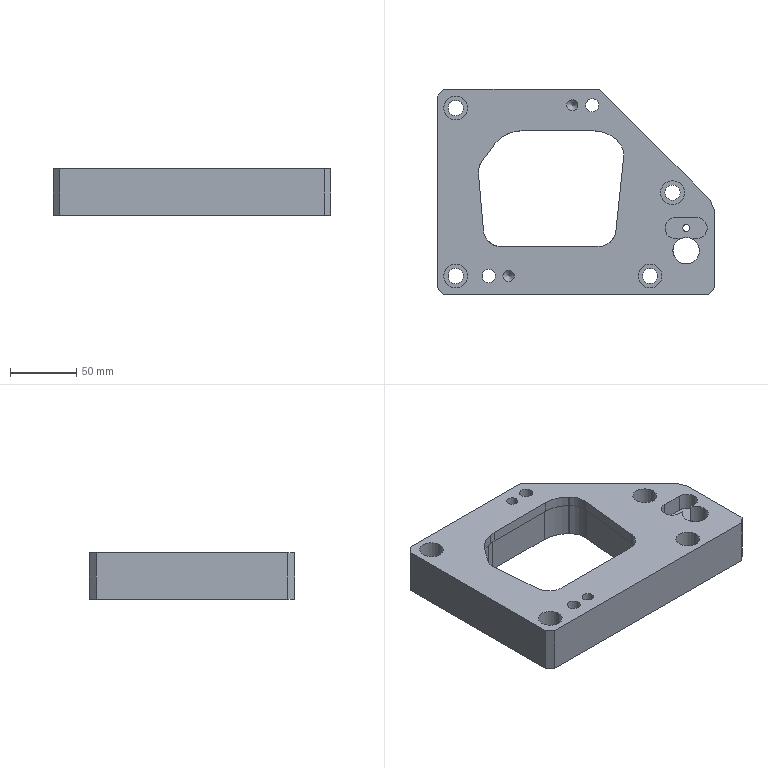Part | STEP file | lll_id202_x_t | 1 solid | 75 faces | box 210 x 155 x 35 mm | volume 629853 mm3 | plane 32 | cylinder 20 | spline 11 | other 10 | cone 2 | commonest cylinder face diameters 11.509 x4 18.008 x4 8.506 x2 10 x2 16 x2 5.206 x1